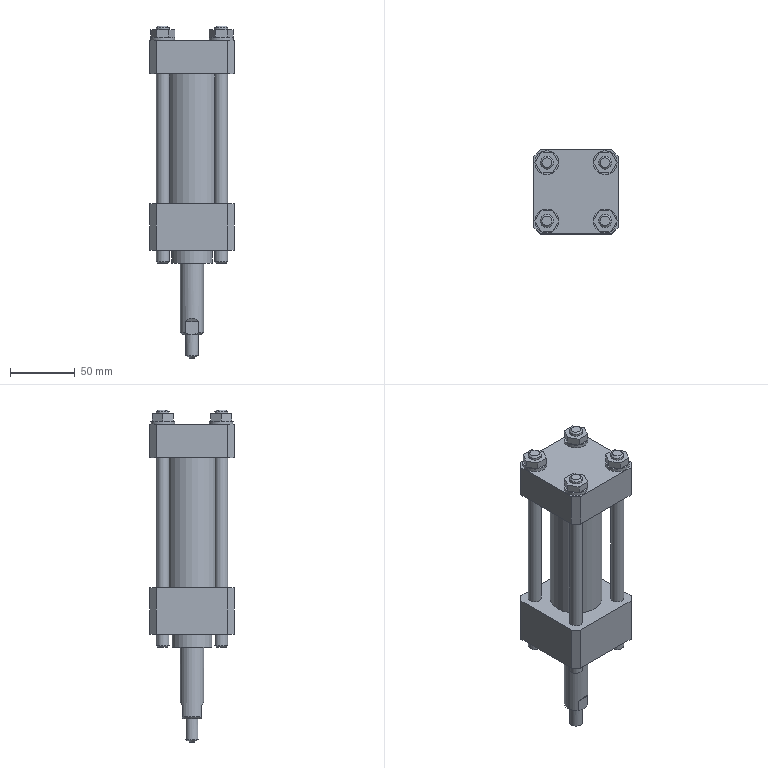Part | STEP file | HYDRAULIC-CYLINDER-2_id478_x_t | 1 solid | 118 faces | box 65 x 65 x 255.997 mm | volume 449957 mm3 | plane 87 | cylinder 20 | cone 11 | commonest cylinder face diameters 10 x13 18.4 x4 18 x1 31 x1 40 x1